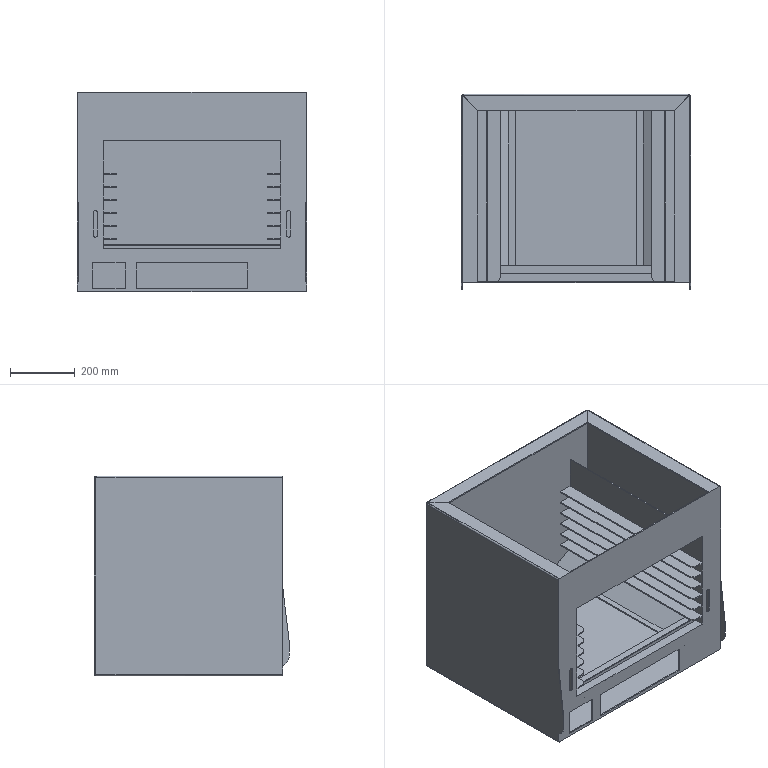Part | SolidWorks | features ICE 10, EdgeFlange 2, Fillet 2, Cut 1, FlatPattern 1, SMBaseFlange 1, SheetMetal 1 | 1 solid | 160 faces | box 706 x 601.439 x 616 mm | volume 10499280 mm3 | plane 119 | cylinder 33 | spline 8 | commonest cylinder face diameters 40 x12 1.473 x6 9.473 x6 12 x6 80 x2 4 x1